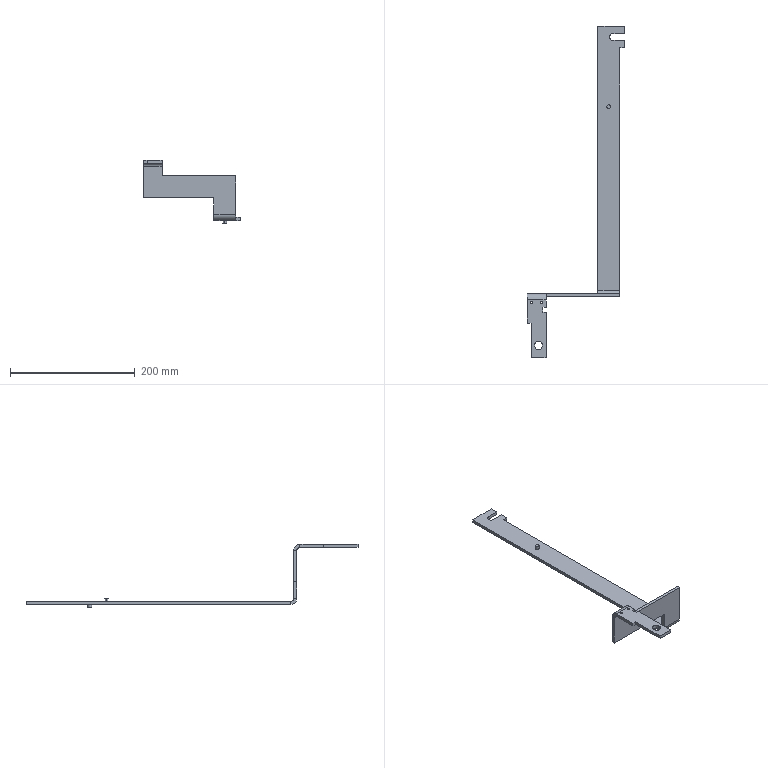Part | STEP file | 64562495 | 1 solid | 52 faces | box 155.9 x 532.25 x 101.5 mm | volume 122513 mm3 | plane 37 | cylinder 15 | commonest cylinder face diameters 4 x4 6 x4 10 x2 12 x2 20 x2 11 x1